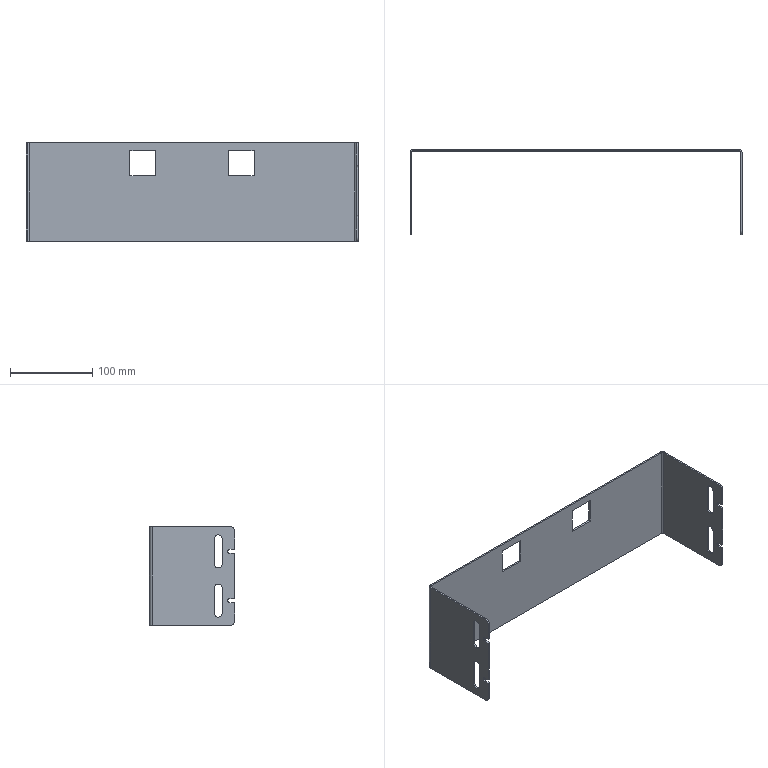Part | NX | 1 solid | 66 faces | box 404 x 104 x 120 mm | volume 138068 mm3 | plane 46 | cylinder 20 | commonest cylinder face diameters 10 x12 5 x4 4 x2 8 x2